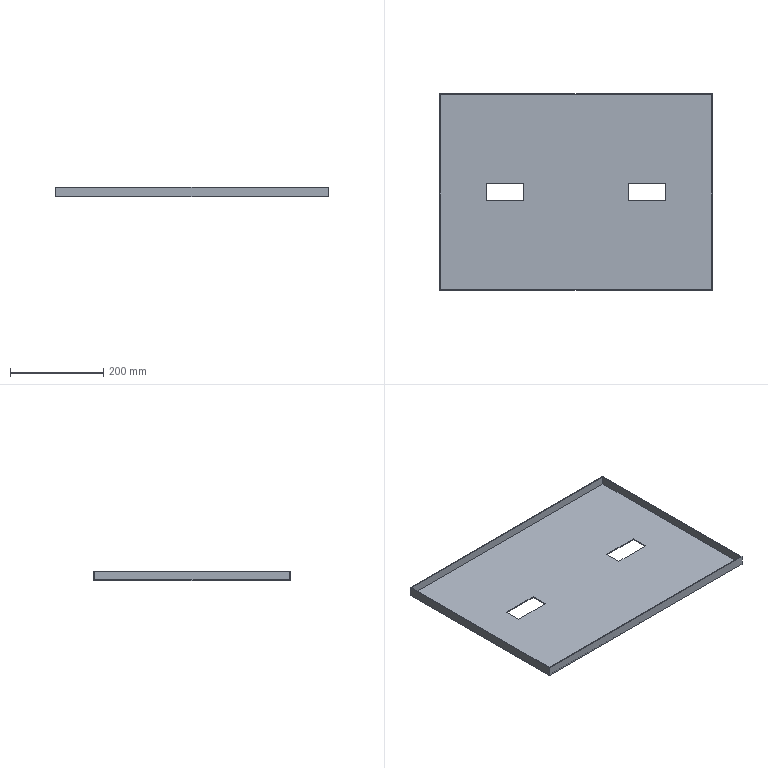Part | STEP file | Side sealing plate | 1 solid | 19 faces | box 585 x 421.75 x 20 mm | volume 553657 mm3 | plane 19
STEP:
#1=CARTESIAN_POINT('',(0.,0.,0.));
#2=DIRECTION('',(0.,0.,1.));
#3=DIRECTION('',(1.,0.,0.));
#4=AXIS2_PLACEMENT_3D('',#1,#2,#3);
#5=CARTESIAN_POINT('',(-292.5,-210.875,0.));
#6=VERTEX_POINT('',#5);
#7=CARTESIAN_POINT('',(292.5,-210.875,0.));
#8=VERTEX_POINT('',#7);
#9=CARTESIAN_POINT('',(0.,-210.875,0.));
#10=DIRECTION('',(1.,0.,0.));
#11=VECTOR('',#10,1.);
#12=LINE('',#9,#11);
#13=CARTESIAN_POINT('',(0.,0.,0.));
#14=DIRECTION('',(0.,0.,1.));
#15=DIRECTION('',(1.,0.,0.));
#16=AXIS2_PLACEMENT_3D('',#13,#14,#15);
#17=PLANE('',#16);
#18=CARTESIAN_POINT('',(0.,-210.875));
#19=DIRECTION('',(1.,0.));
#20=VECTOR('',#19,1.);
#21=LINE('',#18,#20);
#22=(GEOMETRIC_REPRESENTATION_CONTEXT(2)PARAMETRIC_REPRESENTATION_CONTEXT()REPRESENTATION_CONTEXT('',''));
#23=DEFINITIONAL_REPRESENTATION('',(#21),#22);
#24=PCURVE('',#17,#23);
#25=CARTESIAN_POINT('',(-292.5,-210.875,20.));
#26=DIRECTION('',(0.,1.,0.));
#27=DIRECTION('',(0.,0.,1.));
#28=AXIS2_PLACEMENT_3D('',#25,#26,#27);
#29=PLANE('',#28);
#30=CARTESIAN_POINT('',(-20.,292.5));
#31=DIRECTION('',(0.,1.));
#32=VECTOR('',#31,1.);
#33=LINE('',#30,#32);
#34=(GEOMETRIC_REPRESENTATION_CONTEXT(2)PARAMETRIC_REPRESENTATION_CONTEXT()REPRESENTATION_CONTEXT('',''));
#35=DEFINITIONAL_REPRESENTATION('',(#33),#34);
#36=PCURVE('',#29,#35);
#37=SURFACE_CURVE('',#12,(#24,#36),.PCURVE_S1.);
#38=EDGE_CURVE('',#6,#8,#37,.T.);
#39=ORIENTED_EDGE('',*,*,#38,.F.);
#40=CARTESIAN_POINT('',(-292.5,210.875,0.));
#41=VERTEX_POINT('',#40);
#42=CARTESIAN_POINT('',(-292.5,0.,0.));
#43=DIRECTION('',(0.,-1.,0.));
#44=VECTOR('',#43,1.);
#45=LINE('',#42,#44);
#46=CARTESIAN_POINT('',(-292.5,0.));
#47=DIRECTION('',(0.,-1.));
#48=VECTOR('',#47,1.);
#49=LINE('',#46,#48);
#50=(GEOMETRIC_REPRESENTATION_CONTEXT(2)PARAMETRIC_REPRESENTATION_CONTEXT()REPRESENTATION_CONTEXT('',''));
#51=DEFINITIONAL_REPRESENTATION('',(#49),#50);
#52=PCURVE('',#17,#51);
#53=CARTESIAN_POINT('',(-292.5,210.875,20.));
#54=DIRECTION('',(1.,0.,0.));
#55=DIRECTION('',(0.,1.,0.));
#56=AXIS2_PLACEMENT_3D('',#53,#54,#55);
#57=PLANE('',#56);
#58=CARTESIAN_POINT('',(-210.875,-20.));
#59=DIRECTION('',(-1.,0.));
#60=VECTOR('',#59,1.);
#61=LINE('',#58,#60);
#62=(GEOMETRIC_REPRESENTATION_CONTEXT(2)PARAMETRIC_REPRESENTATION_CONTEXT()REPRESENTATION_CONTEXT('',''));
#63=DEFINITIONAL_REPRESENTATION('',(#61),#62);
#64=PCURVE('',#57,#63);
#65=SURFACE_CURVE('',#45,(#52,#64),.PCURVE_S1.);
#66=EDGE_CURVE('',#41,#6,#65,.T.);
#67=ORIENTED_EDGE('',*,*,#66,.F.);
#68=CARTESIAN_POINT('',(292.5,210.875,0.));
#69=VERTEX_POINT('',#68);
#70=CARTESIAN_POINT('',(0.,210.875,0.));
#71=DIRECTION('',(-1.,0.,0.));
#72=VECTOR('',#71,1.);
#73=LINE('',#70,#72);
#74=CARTESIAN_POINT('',(0.,210.875));
#75=DIRECTION('',(-1.,0.));
#76=VECTOR('',#75,1.);
#77=LINE('',#74,#76);
#78=(GEOMETRIC_REPRESENTATION_CONTEXT(2)PARAMETRIC_REPRESENTATION_CONTEXT()REPRESENTATION_CONTEXT('',''));
#79=DEFINITIONAL_REPRESENTATION('',(#77),#78);
#80=PCURVE('',#17,#79);
#81=CARTESIAN_POINT('',(-292.5,210.875,20.));
#82=DIRECTION('',(0.,-1.,0.));
#83=DIRECTION('',(0.,0.,-1.));
#84=AXIS2_PLACEMENT_3D('',#81,#82,#83);
#85=PLANE('',#84);
#86=CARTESIAN_POINT('',(20.,292.5));
#87=DIRECTION('',(0.,-1.));
#88=VECTOR('',#87,1.);
#89=LINE('',#86,#88);
#90=(GEOMETRIC_REPRESENTATION_CONTEXT(2)PARAMETRIC_REPRESENTATION_CONTEXT()REPRESENTATION_CONTEXT('',''));
#91=DEFINITIONAL_REPRESENTATION('',(#89),#90);
#92=PCURVE('',#85,#91);
#93=SURFACE_CURVE('',#73,(#80,#92),.PCURVE_S1.);
#94=EDGE_CURVE('',#69,#41,#93,.T.);
#95=ORIENTED_EDGE('',*,*,#94,.F.);
#96=CARTESIAN_POINT('',(292.5,0.,0.));
#97=DIRECTION('',(0.,1.,0.));
#98=VECTOR('',#97,1.);
#99=LINE('',#96,#98);
#100=CARTESIAN_POINT('',(292.5,0.));
#101=DIRECTION('',(0.,1.));
#102=VECTOR('',#101,1.);
#103=LINE('',#100,#102);
#104=(GEOMETRIC_REPRESENTATION_CONTEXT(2)PARAMETRIC_REPRESENTATION_CONTEXT()REPRESENTATION_CONTEXT('',''));
#105=DEFINITIONAL_REPRESENTATION('',(#103),#104);
#106=PCURVE('',#17,#105);
#107=CARTESIAN_POINT('',(292.5,210.875,20.));
#108=DIRECTION('',(-1.,0.,0.));
#109=DIRECTION('',(0.,-1.,0.));
#110=AXIS2_PLACEMENT_3D('',#107,#108,#109);
#111=PLANE('',#110);
#112=CARTESIAN_POINT('',(210.875,-20.));
#113=DIRECTION('',(-1.,0.));
#114=VECTOR('',#113,1.);
#115=LINE('',#112,#114);
#116=(GEOMETRIC_REPRESENTATION_CONTEXT(2)PARAMETRIC_REPRESENTATION_CONTEXT()REPRESENTATION_CONTEXT('',''));
#117=DEFINITIONAL_REPRESENTATION('',(#115),#116);
#118=PCURVE('',#111,#117);
#119=SURFACE_CURVE('',#99,(#106,#118),.PCURVE_S1.);
#120=EDGE_CURVE('',#8,#69,#119,.T.);
#121=ORIENTED_EDGE('',*,*,#120,.F.);
#122=EDGE_LOOP('',(#39,#67,#95,#121));
#123=FACE_BOUND('',#122,.T.);
#124=CARTESIAN_POINT('',(111.5,-18.5,0.));
#125=VERTEX_POINT('',#124);
#126=CARTESIAN_POINT('',(111.5,18.5,0.));
#127=VERTEX_POINT('',#126);
#128=CARTESIAN_POINT('',(111.5,0.,0.));
#129=DIRECTION('',(0.,1.,0.));
#130=VECTOR('',#129,1.);
#131=LINE('',#128,#130);
#132=CARTESIAN_POINT('',(111.5,0.));
#133=DIRECTION('',(0.,1.));
#134=VECTOR('',#133,1.);
#135=LINE('',#132,#134);
#136=(GEOMETRIC_REPRESENTATION_CONTEXT(2)PARAMETRIC_REPRESENTATION_CONTEXT()REPRESENTATION_CONTEXT('',''));
#137=DEFINITIONAL_REPRESENTATION('',(#135),#136);
#138=PCURVE('',#17,#137);
#139=CARTESIAN_POINT('',(111.5,18.5,20.));
#140=DIRECTION('',(-1.,0.,0.));
#141=DIRECTION('',(0.,0.,1.));
#142=AXIS2_PLACEMENT_3D('',#139,#140,#141);
#143=PLANE('',#142);
#144=CARTESIAN_POINT('',(-20.,-18.5));
#145=DIRECTION('',(0.,1.));
#146=VECTOR('',#145,1.);
#147=LINE('',#144,#146);
#148=(GEOMETRIC_REPRESENTATION_CONTEXT(2)PARAMETRIC_REPRESENTATION_CONTEXT()REPRESENTATION_CONTEXT('',''));
#149=DEFINITIONAL_REPRESENTATION('',(#147),#148);
#150=PCURVE('',#143,#149);
#151=SURFACE_CURVE('',#131,(#138,#150),.PCURVE_S1.);
#152=EDGE_CURVE('',#125,#127,#151,.T.);
#153=ORIENTED_EDGE('',*,*,#152,.F.);
#154=CARTESIAN_POINT('',(192.5,-18.5,0.));
#155=VERTEX_POINT('',#154);
#156=CARTESIAN_POINT('',(0.,-18.5,0.));
#157=DIRECTION('',(-1.,0.,0.));
#158=VECTOR('',#157,1.);
#159=LINE('',#156,#158);
#160=CARTESIAN_POINT('',(0.,-18.5));
#161=DIRECTION('',(-1.,0.));
#162=VECTOR('',#161,1.);
#163=LINE('',#160,#162);
#164=(GEOMETRIC_REPRESENTATION_CONTEXT(2)PARAMETRIC_REPRESENTATION_CONTEXT()REPRESENTATION_CONTEXT('',''));
#165=DEFINITIONAL_REPRESENTATION('',(#163),#164);
#166=PCURVE('',#17,#165);
#167=CARTESIAN_POINT('',(192.5,-18.5,20.));
#168=DIRECTION('',(0.,-1.,0.));
#169=DIRECTION('',(0.,0.,-1.));
#170=AXIS2_PLACEMENT_3D('',#167,#168,#169);
#171=PLANE('',#170);
#172=CARTESIAN_POINT('',(20.,-192.5));
#173=DIRECTION('',(0.,-1.));
#174=VECTOR('',#173,1.);
#175=LINE('',#172,#174);
#176=(GEOMETRIC_REPRESENTATION_CONTEXT(2)PARAMETRIC_REPRESENTATION_CONTEXT()REPRESENTATION_CONTEXT('',''));
#177=DEFINITIONAL_REPRESENTATION('',(#175),#176);
#178=PCURVE('',#171,#177);
#179=SURFACE_CURVE('',#159,(#166,#178),.PCURVE_S1.);
#180=EDGE_CURVE('',#155,#125,#179,.T.);
#181=ORIENTED_EDGE('',*,*,#180,.F.);
#182=CARTESIAN_POINT('',(192.5,18.5,0.));
#183=VERTEX_POINT('',#182);
#184=CARTESIAN_POINT('',(192.5,0.,0.));
#185=DIRECTION('',(0.,-1.,0.));
#186=VECTOR('',#185,1.);
#187=LINE('',#184,#186);
#188=CARTESIAN_POINT('',(192.5,0.));
#189=DIRECTION('',(0.,-1.));
#190=VECTOR('',#189,1.);
#191=LINE('',#188,#190);
#192=(GEOMETRIC_REPRESENTATION_CONTEXT(2)PARAMETRIC_REPRESENTATION_CONTEXT()REPRESENTATION_CONTEXT('',''));
#193=DEFINITIONAL_REPRESENTATION('',(#191),#192);
#194=PCURVE('',#17,#193);
#195=CARTESIAN_POINT('',(192.5,18.5,20.));
#196=DIRECTION('',(1.,0.,0.));
#197=DIRECTION('',(0.,1.,0.));
#198=AXIS2_PLACEMENT_3D('',#195,#196,#197);
#199=PLANE('',#198);
#200=CARTESIAN_POINT('',(-18.5,-20.));
#201=DIRECTION('',(-1.,0.));
#202=VECTOR('',#201,1.);
#203=LINE('',#200,#202);
#204=(GEOMETRIC_REPRESENTATION_CONTEXT(2)PARAMETRIC_REPRESENTATION_CONTEXT()REPRESENTATION_CONTEXT('',''));
#205=DEFINITIONAL_REPRESENTATION('',(#203),#204);
#206=PCURVE('',#199,#205);
#207=SURFACE_CURVE('',#187,(#194,#206),.PCURVE_S1.);
#208=EDGE_CURVE('',#183,#155,#207,.T.);
#209=ORIENTED_EDGE('',*,*,#208,.F.);
#210=CARTESIAN_POINT('',(0.,18.5,0.));
#211=DIRECTION('',(1.,0.,0.));
#212=VECTOR('',#211,1.);
#213=LINE('',#210,#212);
#214=CARTESIAN_POINT('',(0.,18.5));
#215=DIRECTION('',(1.,0.));
#216=VECTOR('',#215,1.);
#217=LINE('',#214,#216);
#218=(GEOMETRIC_REPRESENTATION_CONTEXT(2)PARAMETRIC_REPRESENTATION_CONTEXT()REPRESENTATION_CONTEXT('',''));
#219=DEFINITIONAL_REPRESENTATION('',(#217),#218);
#220=PCURVE('',#17,#219);
#221=CARTESIAN_POINT('',(192.5,18.5,20.));
#222=DIRECTION('',(0.,1.,0.));
#223=DIRECTION('',(0.,0.,1.));
#224=AXIS2_PLACEMENT_3D('',#221,#222,#223);
#225=PLANE('',#224);
#226=CARTESIAN_POINT('',(-20.,-192.5));
#227=DIRECTION('',(0.,1.));
#228=VECTOR('',#227,1.);
#229=LINE('',#226,#228);
#230=(GEOMETRIC_REPRESENTATION_CONTEXT(2)PARAMETRIC_REPRESENTATION_CONTEXT()REPRESENTATION_CONTEXT('',''));
#231=DEFINITIONAL_REPRESENTATION('',(#229),#230);
#232=PCURVE('',#225,#231);
#233=SURFACE_CURVE('',#213,(#220,#232),.PCURVE_S1.);
#234=EDGE_CURVE('',#127,#183,#233,.T.);
#235=ORIENTED_EDGE('',*,*,#234,.F.);
#236=EDGE_LOOP('',(#153,#181,#209,#235));
#237=FACE_BOUND('',#236,.T.);
#238=CARTESIAN_POINT('',(-192.5,-18.5,0.));
#239=VERTEX_POINT('',#238);
#240=CARTESIAN_POINT('',(-192.5,18.5,0.));
#241=VERTEX_POINT('',#240);
#242=CARTESIAN_POINT('',(-192.5,0.,0.));
#243=DIRECTION('',(0.,1.,0.));
#244=VECTOR('',#243,1.);
#245=LINE('',#242,#244);
#246=CARTESIAN_POINT('',(-192.5,0.));
#247=DIRECTION('',(0.,1.));
#248=VECTOR('',#247,1.);
#249=LINE('',#246,#248);
#250=(GEOMETRIC_REPRESENTATION_CONTEXT(2)PARAMETRIC_REPRESENTATION_CONTEXT()REPRESENTATION_CONTEXT('',''));
#251=DEFINITIONAL_REPRESENTATION('',(#249),#250);
#252=PCURVE('',#17,#251);
#253=CARTESIAN_POINT('',(-192.5,18.5,20.));
#254=DIRECTION('',(-1.,0.,0.));
#255=DIRECTION('',(0.,0.,1.));
#256=AXIS2_PLACEMENT_3D('',#253,#254,#255);
#257=PLANE('',#256);
#258=CARTESIAN_POINT('',(-20.,-18.5));
#259=DIRECTION('',(0.,1.));
#260=VECTOR('',#259,1.);
#261=LINE('',#258,#260);
#262=(GEOMETRIC_REPRESENTATION_CONTEXT(2)PARAMETRIC_REPRESENTATION_CONTEXT()REPRESENTATION_CONTEXT('',''));
#263=DEFINITIONAL_REPRESENTATION('',(#261),#262);
#264=PCURVE('',#257,#263);
#265=SURFACE_CURVE('',#245,(#252,#264),.PCURVE_S1.);
#266=EDGE_CURVE('',#239,#241,#265,.T.);
#267=ORIENTED_EDGE('',*,*,#266,.F.);
#268=CARTESIAN_POINT('',(-111.5,-18.5,0.));
#269=VERTEX_POINT('',#268);
#270=CARTESIAN_POINT('',(0.,-18.5,0.));
#271=DIRECTION('',(-1.,0.,0.));
#272=VECTOR('',#271,1.);
#273=LINE('',#270,#272);
#274=CARTESIAN_POINT('',(0.,-18.5));
#275=DIRECTION('',(-1.,0.));
#276=VECTOR('',#275,1.);
#277=LINE('',#274,#276);
#278=(GEOMETRIC_REPRESENTATION_CONTEXT(2)PARAMETRIC_REPRESENTATION_CONTEXT()REPRESENTATION_CONTEXT('',''));
#279=DEFINITIONAL_REPRESENTATION('',(#277),#278);
#280=PCURVE('',#17,#279);
#281=CARTESIAN_POINT('',(-111.5,-18.5,20.));
#282=DIRECTION('',(0.,-1.,0.));
#283=DIRECTION('',(0.,0.,-1.));
#284=AXIS2_PLACEMENT_3D('',#281,#282,#283);
#285=PLANE('',#284);
#286=CARTESIAN_POINT('',(20.,111.5));
#287=DIRECTION('',(0.,-1.));
#288=VECTOR('',#287,1.);
#289=LINE('',#286,#288);
#290=(GEOMETRIC_REPRESENTATION_CONTEXT(2)PARAMETRIC_REPRESENTATION_CONTEXT()REPRESENTATION_CONTEXT('',''));
#291=DEFINITIONAL_REPRESENTATION('',(#289),#290);
#292=PCURVE('',#285,#291);
#293=SURFACE_CURVE('',#273,(#280,#292),.PCURVE_S1.);
#294=EDGE_CURVE('',#269,#239,#293,.T.);
#295=ORIENTED_EDGE('',*,*,#294,.F.);
#296=CARTESIAN_POINT('',(-111.5,18.5,0.));
#297=VERTEX_POINT('',#296);
#298=CARTESIAN_POINT('',(-111.5,0.,0.));
#299=DIRECTION('',(0.,-1.,0.));
#300=VECTOR('',#299,1.);
#301=LINE('',#298,#300);
#302=CARTESIAN_POINT('',(-111.5,0.));
#303=DIRECTION('',(0.,-1.));
#304=VECTOR('',#303,1.);
#305=LINE('',#302,#304);
#306=(GEOMETRIC_REPRESENTATION_CONTEXT(2)PARAMETRIC_REPRESENTATION_CONTEXT()REPRESENTATION_CONTEXT('',''));
#307=DEFINITIONAL_REPRESENTATION('',(#305),#306);
#308=PCURVE('',#17,#307);
#309=CARTESIAN_POINT('',(-111.5,18.5,20.));
#310=DIRECTION('',(1.,0.,0.));
#311=DIRECTION('',(0.,0.,-1.));
#312=AXIS2_PLACEMENT_3D('',#309,#310,#311);
#313=PLANE('',#312);
#314=CARTESIAN_POINT('',(20.,-18.5));
#315=DIRECTION('',(0.,-1.));
#316=VECTOR('',#315,1.);
#317=LINE('',#314,#316);
#318=(GEOMETRIC_REPRESENTATION_CONTEXT(2)PARAMETRIC_REPRESENTATION_CONTEXT()REPRESENTATION_CONTEXT('',''));
#319=DEFINITIONAL_REPRESENTATION('',(#317),#318);
#320=PCURVE('',#313,#319);
#321=SURFACE_CURVE('',#301,(#308,#320),.PCURVE_S1.);
#322=EDGE_CURVE('',#297,#269,#321,.T.);
#323=ORIENTED_EDGE('',*,*,#322,.F.);
#324=CARTESIAN_POINT('',(0.,18.5,0.));
#325=DIRECTION('',(1.,0.,0.));
#326=VECTOR('',#325,1.);
#327=LINE('',#324,#326);
#328=CARTESIAN_POINT('',(0.,18.5));
#329=DIRECTION('',(1.,0.));
#330=VECTOR('',#329,1.);
#331=LINE('',#328,#330);
#332=(GEOMETRIC_REPRESENTATION_CONTEXT(2)PARAMETRIC_REPRESENTATION_CONTEXT()REPRESENTATION_CONTEXT('',''));
#333=DEFINITIONAL_REPRESENTATION('',(#331),#332);
#334=PCURVE('',#17,#333);
#335=CARTESIAN_POINT('',(-111.5,18.5,20.));
#336=DIRECTION('',(0.,1.,0.));
#337=DIRECTION('',(-1.,0.,0.));
#338=AXIS2_PLACEMENT_3D('',#335,#336,#337);
#339=PLANE('',#338);
#340=CARTESIAN_POINT('',(-111.5,-20.));
#341=DIRECTION('',(-1.,0.));
#342=VECTOR('',#341,1.);
#343=LINE('',#340,#342);
#344=(GEOMETRIC_REPRESENTATION_CONTEXT(2)PARAMETRIC_REPRESENTATION_CONTEXT()REPRESENTATION_CONTEXT('',''));
#345=DEFINITIONAL_REPRESENTATION('',(#343),#344);
#346=PCURVE('',#339,#345);
#347=SURFACE_CURVE('',#327,(#334,#346),.PCURVE_S1.);
#348=EDGE_CURVE('',#241,#297,#347,.T.);
#349=ORIENTED_EDGE('',*,*,#348,.F.);
#350=EDGE_LOOP('',(#267,#295,#323,#349));
#351=FACE_BOUND('',#350,.T.);
#352=ADVANCED_FACE('',(#123,#237,#351),#17,.F.);
#353=CARTESIAN_POINT('',(292.5,210.875,20.));
#354=VERTEX_POINT('',#353);
#355=CARTESIAN_POINT('',(292.5,210.875,20.));
#356=DIRECTION('',(0.,0.,-1.));
#357=VECTOR('',#356,1.);
#358=LINE('',#355,#357);
#359=CARTESIAN_POINT('',(0.,0.));
#360=DIRECTION('',(0.,-1.));
#361=VECTOR('',#360,1.);
#362=LINE('',#359,#361);
#363=(GEOMETRIC_REPRESENTATION_CONTEXT(2)PARAMETRIC_REPRESENTATION_CONTEXT()REPRESENTATION_CONTEXT('',''));
#364=DEFINITIONAL_REPRESENTATION('',(#362),#363);
#365=PCURVE('',#111,#364);
#366=CARTESIAN_POINT('',(0.,585.));
#367=DIRECTION('',(1.,0.));
#368=VECTOR('',#367,1.);
#369=LINE('',#366,#368);
#370=(GEOMETRIC_REPRESENTATION_CONTEXT(2)PARAMETRIC_REPRESENTATION_CONTEXT()REPRESENTATION_CONTEXT('',''));
#371=DEFINITIONAL_REPRESENTATION('',(#369),#370);
#372=PCURVE('',#85,#371);
#373=SURFACE_CURVE('',#358,(#365,#372),.PCURVE_S1.);
#374=EDGE_CURVE('',#354,#69,#373,.T.);
#375=ORIENTED_EDGE('',*,*,#374,.F.);
#376=CARTESIAN_POINT('',(292.5,-210.875,20.));
#377=VERTEX_POINT('',#376);
#378=CARTESIAN_POINT('',(292.5,210.875,20.));
#379=DIRECTION('',(0.,1.,0.));
#380=VECTOR('',#379,1.);
#381=LINE('',#378,#380);
#382=CARTESIAN_POINT('',(0.,0.));
#383=DIRECTION('',(-1.,0.));
#384=VECTOR('',#383,1.);
#385=LINE('',#382,#384);
#386=(GEOMETRIC_REPRESENTATION_CONTEXT(2)PARAMETRIC_REPRESENTATION_CONTEXT()REPRESENTATION_CONTEXT('',''));
#387=DEFINITIONAL_REPRESENTATION('',(#385),#386);
#388=PCURVE('',#111,#387);
#389=CARTESIAN_POINT('',(0.,0.,20.));
#390=DIRECTION('',(0.,0.,1.));
#391=DIRECTION('',(1.,0.,0.));
#392=AXIS2_PLACEMENT_3D('',#389,#390,#391);
#393=PLANE('',#392);
#394=CARTESIAN_POINT('',(292.5,210.875));
#395=DIRECTION('',(0.,1.));
#396=VECTOR('',#395,1.);
#397=LINE('',#394,#396);
#398=(GEOMETRIC_REPRESENTATION_CONTEXT(2)PARAMETRIC_REPRESENTATION_CONTEXT()REPRESENTATION_CONTEXT('',''));
#399=DEFINITIONAL_REPRESENTATION('',(#397),#398);
#400=PCURVE('',#393,#399);
#401=SURFACE_CURVE('',#381,(#388,#400),.PCURVE_S1.);
#402=EDGE_CURVE('',#377,#354,#401,.T.);
#403=ORIENTED_EDGE('',*,*,#402,.F.);
#404=CARTESIAN_POINT('',(292.5,-210.875,20.));
#405=DIRECTION('',(0.,0.,1.));
#406=VECTOR('',#405,1.);
#407=LINE('',#404,#406);
#408=CARTESIAN_POINT('',(421.75,0.));
#409=DIRECTION('',(0.,1.));
#410=VECTOR('',#409,1.);
#411=LINE('',#408,#410);
#412=(GEOMETRIC_REPRESENTATION_CONTEXT(2)PARAMETRIC_REPRESENTATION_CONTEXT()REPRESENTATION_CONTEXT('',''));
#413=DEFINITIONAL_REPRESENTATION('',(#411),#412);
#414=PCURVE('',#111,#413);
#415=CARTESIAN_POINT('',(0.,585.));
#416=DIRECTION('',(1.,0.));
#417=VECTOR('',#416,1.);
#418=LINE('',#415,#417);
#419=(GEOMETRIC_REPRESENTATION_CONTEXT(2)PARAMETRIC_REPRESENTATION_CONTEXT()REPRESENTATION_CONTEXT('',''));
#420=DEFINITIONAL_REPRESENTATION('',(#418),#419);
#421=PCURVE('',#29,#420);
#422=SURFACE_CURVE('',#407,(#414,#421),.PCURVE_S1.);
#423=EDGE_CURVE('',#8,#377,#422,.T.);
#424=ORIENTED_EDGE('',*,*,#423,.F.);
#425=ORIENTED_EDGE('',*,*,#120,.T.);
#426=EDGE_LOOP('',(#375,#403,#424,#425));
#427=FACE_BOUND('',#426,.T.);
#428=ADVANCED_FACE('',(#427),#111,.F.);
#429=ORIENTED_EDGE('',*,*,#423,.T.);
#430=CARTESIAN_POINT('',(-292.5,-210.875,20.));
#431=VERTEX_POINT('',#430);
#432=CARTESIAN_POINT('',(-292.5,-210.875,20.));
#433=DIRECTION('',(1.,0.,0.));
#434=VECTOR('',#433,1.);
#435=LINE('',#432,#434);
#436=CARTESIAN_POINT('',(0.,0.));
#437=DIRECTION('',(0.,1.));
#438=VECTOR('',#437,1.);
#439=LINE('',#436,#438);
#440=(GEOMETRIC_REPRESENTATION_CONTEXT(2)PARAMETRIC_REPRESENTATION_CONTEXT()REPRESENTATION_CONTEXT('',''));
#441=DEFINITIONAL_REPRESENTATION('',(#439),#440);
#442=PCURVE('',#29,#441);
#443=CARTESIAN_POINT('',(-292.5,-210.875));
#444=DIRECTION('',(1.,0.));
#445=VECTOR('',#444,1.);
#446=LINE('',#443,#445);
#447=(GEOMETRIC_REPRESENTATION_CONTEXT(2)PARAMETRIC_REPRESENTATION_CONTEXT()REPRESENTATION_CONTEXT('',''));
#448=DEFINITIONAL_REPRESENTATION('',(#446),#447);
#449=PCURVE('',#393,#448);
#450=SURFACE_CURVE('',#435,(#442,#449),.PCURVE_S1.);
#451=EDGE_CURVE('',#431,#377,#450,.T.);
#452=ORIENTED_EDGE('',*,*,#451,.F.);
#453=CARTESIAN_POINT('',(-292.5,-210.875,20.));
#454=DIRECTION('',(0.,0.,1.));
#455=VECTOR('',#454,1.);
#456=LINE('',#453,#455);
#457=CARTESIAN_POINT('',(0.,0.));
#458=DIRECTION('',(1.,0.));
#459=VECTOR('',#458,1.);
#460=LINE('',#457,#459);
#461=(GEOMETRIC_REPRESENTATION_CONTEXT(2)PARAMETRIC_REPRESENTATION_CONTEXT()REPRESENTATION_CONTEXT('',''));
#462=DEFINITIONAL_REPRESENTATION('',(#460),#461);
#463=PCURVE('',#29,#462);
#464=CARTESIAN_POINT('',(-421.75,0.));
#465=DIRECTION('',(0.,1.));
#466=VECTOR('',#465,1.);
#467=LINE('',#464,#466);
#468=(GEOMETRIC_REPRESENTATION_CONTEXT(2)PARAMETRIC_REPRESENTATION_CONTEXT()REPRESENTATION_CONTEXT('',''));
#469=DEFINITIONAL_REPRESENTATION('',(#467),#468);
#470=PCURVE('',#57,#469);
#471=SURFACE_CURVE('',#456,(#463,#470),.PCURVE_S1.);
#472=EDGE_CURVE('',#6,#431,#471,.T.);
#473=ORIENTED_EDGE('',*,*,#472,.F.);
#474=ORIENTED_EDGE('',*,*,#38,.T.);
#475=EDGE_LOOP('',(#429,#452,#473,#474));
#476=FACE_BOUND('',#475,.T.);
#477=ADVANCED_FACE('',(#476),#29,.F.);
#478=ORIENTED_EDGE('',*,*,#472,.T.);
#479=CARTESIAN_POINT('',(-292.5,210.875,20.));
#480=VERTEX_POINT('',#479);
#481=CARTESIAN_POINT('',(-292.5,210.875,20.));
#482=DIRECTION('',(0.,-1.,0.));
#483=VECTOR('',#482,1.);
#484=LINE('',#481,#483);
#485=CARTESIAN_POINT('',(0.,0.));
#486=DIRECTION('',(-1.,0.));
#487=VECTOR('',#486,1.);
#488=LINE('',#485,#487);
#489=(GEOMETRIC_REPRESENTATION_CONTEXT(2)PARAMETRIC_REPRESENTATION_CONTEXT()REPRESENTATION_CONTEXT('',''));
#490=DEFINITIONAL_REPRESENTATION('',(#488),#489);
#491=PCURVE('',#57,#490);
#492=CARTESIAN_POINT('',(-292.5,210.875));
#493=DIRECTION('',(0.,-1.));
#494=VECTOR('',#493,1.);
#495=LINE('',#492,#494);
#496=(GEOMETRIC_REPRESENTATION_CONTEXT(2)PARAMETRIC_REPRESENTATION_CONTEXT()REPRESENTATION_CONTEXT('',''));
#497=DEFINITIONAL_REPRESENTATION('',(#495),#496);
#498=PCURVE('',#393,#497);
#499=SURFACE_CURVE('',#484,(#491,#498),.PCURVE_S1.);
#500=EDGE_CURVE('',#480,#431,#499,.T.);
#501=ORIENTED_EDGE('',*,*,#500,.F.);
#502=CARTESIAN_POINT('',(-292.5,210.875,20.));
#503=DIRECTION('',(0.,0.,1.));
#504=VECTOR('',#503,1.);
#505=LINE('',#502,#504);
#506=CARTESIAN_POINT('',(0.,0.));
#507=DIRECTION('',(0.,1.));
#508=VECTOR('',#507,1.);
#509=LINE('',#506,#508);
#510=(GEOMETRIC_REPRESENTATION_CONTEXT(2)PARAMETRIC_REPRESENTATION_CONTEXT()REPRESENTATION_CONTEXT('',''));
#511=DEFINITIONAL_REPRESENTATION('',(#509),#510);
#512=PCURVE('',#57,#511);
#513=CARTESIAN_POINT('',(0.,0.));
#514=DIRECTION('',(-1.,0.));
#515=VECTOR('',#514,1.);
#516=LINE('',#513,#515);
#517=(GEOMETRIC_REPRESENTATION_CONTEXT(2)PARAMETRIC_REPRESENTATION_CONTEXT()REPRESENTATION_CONTEXT('',''));
#518=DEFINITIONAL_REPRESENTATION('',(#516),#517);
#519=PCURVE('',#85,#518);
#520=SURFACE_CURVE('',#505,(#512,#519),.PCURVE_S1.);
#521=EDGE_CURVE('',#41,#480,#520,.T.);
#522=ORIENTED_EDGE('',*,*,#521,.F.);
#523=ORIENTED_EDGE('',*,*,#66,.T.);
#524=EDGE_LOOP('',(#478,#501,#522,#523));
#525=FACE_BOUND('',#524,.T.);
#526=ADVANCED_FACE('',(#525),#57,.F.);
#527=ORIENTED_EDGE('',*,*,#521,.T.);
#528=CARTESIAN_POINT('',(-292.5,210.875,20.));
#529=DIRECTION('',(-1.,0.,0.));
#530=VECTOR('',#529,1.);
#531=LINE('',#528,#530);
#532=CARTESIAN_POINT('',(0.,0.));
#533=DIRECTION('',(0.,-1.));
#534=VECTOR('',#533,1.);
#535=LINE('',#532,#534);
#536=(GEOMETRIC_REPRESENTATION_CONTEXT(2)PARAMETRIC_REPRESENTATION_CONTEXT()REPRESENTATION_CONTEXT('',''));
#537=DEFINITIONAL_REPRESENTATION('',(#535),#536);
#538=PCURVE('',#85,#537);
#539=CARTESIAN_POINT('',(-292.5,210.875));
#540=DIRECTION('',(-1.,0.));
#541=VECTOR('',#540,1.);
#542=LINE('',#539,#541);
#543=(GEOMETRIC_REPRESENTATION_CONTEXT(2)PARAMETRIC_REPRESENTATION_CONTEXT()REPRESENTATION_CONTEXT('',''));
#544=DEFINITIONAL_REPRESENTATION('',(#542),#543);
#545=PCURVE('',#393,#544);
#546=SURFACE_CURVE('',#531,(#538,#545),.PCURVE_S1.);
#547=EDGE_CURVE('',#354,#480,#546,.T.);
#548=ORIENTED_EDGE('',*,*,#547,.F.);
#549=ORIENTED_EDGE('',*,*,#374,.T.);
#550=ORIENTED_EDGE('',*,*,#94,.T.);
#551=EDGE_LOOP('',(#527,#548,#549,#550));
#552=FACE_BOUND('',#551,.T.);
#553=ADVANCED_FACE('',(#552),#85,.F.);
#554=CARTESIAN_POINT('',(111.5,18.5,2.));
#555=VERTEX_POINT('',#554);
#556=CARTESIAN_POINT('',(111.5,18.5,20.));
#557=DIRECTION('',(0.,0.,1.));
#558=VECTOR('',#557,1.);
#559=LINE('',#556,#558);
#560=CARTESIAN_POINT('',(0.,-81.));
#561=DIRECTION('',(1.,0.));
#562=VECTOR('',#561,1.);
#563=LINE('',#560,#562);
#564=(GEOMETRIC_REPRESENTATION_CONTEXT(2)PARAMETRIC_REPRESENTATION_CONTEXT()REPRESENTATION_CONTEXT('',''));
#565=DEFINITIONAL_REPRESENTATION('',(#563),#564);
#566=PCURVE('',#225,#565);
#567=CARTESIAN_POINT('',(0.,0.));
#568=DIRECTION('',(1.,0.));
#569=VECTOR('',#568,1.);
#570=LINE('',#567,#569);
#571=(GEOMETRIC_REPRESENTATION_CONTEXT(2)PARAMETRIC_REPRESENTATION_CONTEXT()REPRESENTATION_CONTEXT('',''));
#572=DEFINITIONAL_REPRESENTATION('',(#570),#571);
#573=PCURVE('',#143,#572);
#574=SURFACE_CURVE('',#559,(#566,#573),.PCURVE_S1.);
#575=EDGE_CURVE('',#127,#555,#574,.T.);
#576=ORIENTED_EDGE('',*,*,#575,.F.);
#577=ORIENTED_EDGE('',*,*,#234,.T.);
#578=CARTESIAN_POINT('',(192.5,18.5,2.));
#579=VERTEX_POINT('',#578);
#580=CARTESIAN_POINT('',(192.5,18.5,20.));
#581=DIRECTION('',(0.,0.,-1.));
#582=VECTOR('',#581,1.);
#583=LINE('',#580,#582);
#584=CARTESIAN_POINT('',(0.,0.));
#585=DIRECTION('',(-1.,0.));
#586=VECTOR('',#585,1.);
#587=LINE('',#584,#586);
#588=(GEOMETRIC_REPRESENTATION_CONTEXT(2)PARAMETRIC_REPRESENTATION_CONTEXT()REPRESENTATION_CONTEXT('',''));
#589=DEFINITIONAL_REPRESENTATION('',(#587),#588);
#590=PCURVE('',#225,#589);
#591=CARTESIAN_POINT('',(0.,0.));
#592=DIRECTION('',(0.,-1.));
#593=VECTOR('',#592,1.);
#594=LINE('',#591,#593);
#595=(GEOMETRIC_REPRESENTATION_CONTEXT(2)PARAMETRIC_REPRESENTATION_CONTEXT()REPRESENTATION_CONTEXT('',''));
#596=DEFINITIONAL_REPRESENTATION('',(#594),#595);
#597=PCURVE('',#199,#596);
#598=SURFACE_CURVE('',#583,(#590,#597),.PCURVE_S1.);
#599=EDGE_CURVE('',#579,#183,#598,.T.);
#600=ORIENTED_EDGE('',*,*,#599,.F.);
#601=CARTESIAN_POINT('',(192.5,18.5,2.));
#602=DIRECTION('',(1.,0.,0.));
#603=VECTOR('',#602,1.);
#604=LINE('',#601,#603);
#605=CARTESIAN_POINT('',(-18.,0.));
#606=DIRECTION('',(0.,1.));
#607=VECTOR('',#606,1.);
#608=LINE('',#605,#607);
#609=(GEOMETRIC_REPRESENTATION_CONTEXT(2)PARAMETRIC_REPRESENTATION_CONTEXT()REPRESENTATION_CONTEXT('',''));
#610=DEFINITIONAL_REPRESENTATION('',(#608),#609);
#611=PCURVE('',#225,#610);
#612=CARTESIAN_POINT('',(0.,0.,2.));
#613=DIRECTION('',(0.,0.,1.));
#614=DIRECTION('',(1.,0.,0.));
#615=AXIS2_PLACEMENT_3D('',#612,#613,#614);
#616=PLANE('',#615);
#617=CARTESIAN_POINT('',(192.5,18.5));
#618=DIRECTION('',(1.,0.));
#619=VECTOR('',#618,1.);
#620=LINE('',#617,#619);
#621=(GEOMETRIC_REPRESENTATION_CONTEXT(2)PARAMETRIC_REPRESENTATION_CONTEXT()REPRESENTATION_CONTEXT('',''));
#622=DEFINITIONAL_REPRESENTATION('',(#620),#621);
#623=PCURVE('',#616,#622);
#624=SURFACE_CURVE('',#604,(#611,#623),.PCURVE_S1.);
#625=EDGE_CURVE('',#555,#579,#624,.T.);
#626=ORIENTED_EDGE('',*,*,#625,.F.);
#627=EDGE_LOOP('',(#576,#577,#600,#626));
#628=FACE_BOUND('',#627,.T.);
#629=ADVANCED_FACE('',(#628),#225,.F.);
#630=CARTESIAN_POINT('',(111.5,-18.5,2.));
#631=VERTEX_POINT('',#630);
#632=CARTESIAN_POINT('',(111.5,-18.5,20.));
#633=DIRECTION('',(0.,0.,1.));
#634=VECTOR('',#633,1.);
#635=LINE('',#632,#634);
#636=CARTESIAN_POINT('',(0.,-37.));
#637=DIRECTION('',(1.,0.));
#638=VECTOR('',#637,1.);
#639=LINE('',#636,#638);
#640=(GEOMETRIC_REPRESENTATION_CONTEXT(2)PARAMETRIC_REPRESENTATION_CONTEXT()REPRESENTATION_CONTEXT('',''));
#641=DEFINITIONAL_REPRESENTATION('',(#639),#640);
#642=PCURVE('',#143,#641);
#643=CARTESIAN_POINT('',(0.,-81.));
#644=DIRECTION('',(-1.,0.));
#645=VECTOR('',#644,1.);
#646=LINE('',#643,#645);
#647=(GEOMETRIC_REPRESENTATION_CONTEXT(2)PARAMETRIC_REPRESENTATION_CONTEXT()REPRESENTATION_CONTEXT('',''));
#648=DEFINITIONAL_REPRESENTATION('',(#646),#647);
#649=PCURVE('',#171,#648);
#650=SURFACE_CURVE('',#635,(#642,#649),.PCURVE_S1.);
#651=EDGE_CURVE('',#125,#631,#650,.T.);
#652=ORIENTED_EDGE('',*,*,#651,.F.);
#653=ORIENTED_EDGE('',*,*,#152,.T.);
#654=ORIENTED_EDGE('',*,*,#575,.T.);
#655=CARTESIAN_POINT('',(111.5,18.5,2.));
#656=DIRECTION('',(0.,1.,0.));
#657=VECTOR('',#656,1.);
#658=LINE('',#655,#657);
#659=CARTESIAN_POINT('',(-18.,0.));
#660=DIRECTION('',(0.,1.));
#661=VECTOR('',#660,1.);
#662=LINE('',#659,#661);
#663=(GEOMETRIC_REPRESENTATION_CONTEXT(2)PARAMETRIC_REPRESENTATION_CONTEXT()REPRESENTATION_CONTEXT('',''));
#664=DEFINITIONAL_REPRESENTATION('',(#662),#663);
#665=PCURVE('',#143,#664);
#666=CARTESIAN_POINT('',(111.5,18.5));
#667=DIRECTION('',(0.,1.));
#668=VECTOR('',#667,1.);
#669=LINE('',#666,#668);
#670=(GEOMETRIC_REPRESENTATION_CONTEXT(2)PARAMETRIC_REPRESENTATION_CONTEXT()REPRESENTATION_CONTEXT('',''));
#671=DEFINITIONAL_REPRESENTATION('',(#669),#670);
#672=PCURVE('',#616,#671);
#673=SURFACE_CURVE('',#658,(#665,#672),.PCURVE_S1.);
#674=EDGE_CURVE('',#631,#555,#673,.T.);
#675=ORIENTED_EDGE('',*,*,#674,.F.);
#676=EDGE_LOOP('',(#652,#653,#654,#675));
#677=FACE_BOUND('',#676,.T.);
#678=ADVANCED_FACE('',(#677),#143,.F.);
#679=CARTESIAN_POINT('',(192.5,-18.5,2.));
#680=VERTEX_POINT('',#679);
#681=CARTESIAN_POINT('',(192.5,-18.5,20.));
#682=DIRECTION('',(0.,0.,1.));
#683=VECTOR('',#682,1.);
#684=LINE('',#681,#683);
#685=CARTESIAN_POINT('',(0.,0.));
#686=DIRECTION('',(-1.,0.));
#687=VECTOR('',#686,1.);
#688=LINE('',#685,#687);
#689=(GEOMETRIC_REPRESENTATION_CONTEXT(2)PARAMETRIC_REPRESENTATION_CONTEXT()REPRESENTATION_CONTEXT('',''));
#690=DEFINITIONAL_REPRESENTATION('',(#688),#689);
#691=PCURVE('',#171,#690);
#692=CARTESIAN_POINT('',(-37.,0.));
#693=DIRECTION('',(0.,1.));
#694=VECTOR('',#693,1.);
#695=LINE('',#692,#694);
#696=(GEOMETRIC_REPRESENTATION_CONTEXT(2)PARAMETRIC_REPRESENTATION_CONTEXT()REPRESENTATION_CONTEXT('',''));
#697=DEFINITIONAL_REPRESENTATION('',(#695),#696);
#698=PCURVE('',#199,#697);
#699=SURFACE_CURVE('',#684,(#691,#698),.PCURVE_S1.);
#700=EDGE_CURVE('',#155,#680,#699,.T.);
#701=ORIENTED_EDGE('',*,*,#700,.F.);
#702=ORIENTED_EDGE('',*,*,#180,.T.);
#703=ORIENTED_EDGE('',*,*,#651,.T.);
#704=CARTESIAN_POINT('',(192.5,-18.5,2.));
#705=DIRECTION('',(-1.,0.,0.));
#706=VECTOR('',#705,1.);
#707=LINE('',#704,#706);
#708=CARTESIAN_POINT('',(18.,0.));
#709=DIRECTION('',(0.,-1.));
#710=VECTOR('',#709,1.);
#711=LINE('',#708,#710);
#712=(GEOMETRIC_REPRESENTATION_CONTEXT(2)PARAMETRIC_REPRESENTATION_CONTEXT()REPRESENTATION_CONTEXT('',''));
#713=DEFINITIONAL_REPRESENTATION('',(#711),#712);
#714=PCURVE('',#171,#713);
#715=CARTESIAN_POINT('',(192.5,-18.5));
#716=DIRECTION('',(-1.,0.));
#717=VECTOR('',#716,1.);
#718=LINE('',#715,#717);
#719=(GEOMETRIC_REPRESENTATION_CONTEXT(2)PARAMETRIC_REPRESENTATION_CONTEXT()REPRESENTATION_CONTEXT('',''));
#720=DEFINITIONAL_REPRESENTATION('',(#718),#719);
#721=PCURVE('',#616,#720);
#722=SURFACE_CURVE('',#707,(#714,#721),.PCURVE_S1.);
#723=EDGE_CURVE('',#680,#631,#722,.T.);
#724=ORIENTED_EDGE('',*,*,#723,.F.);
#725=EDGE_LOOP('',(#701,#702,#703,#724));
#726=FACE_BOUND('',#725,.T.);
#727=ADVANCED_FACE('',(#726),#171,.F.);
#728=ORIENTED_EDGE('',*,*,#599,.T.);
#729=ORIENTED_EDGE('',*,*,#208,.T.);
#730=ORIENTED_EDGE('',*,*,#700,.T.);
#731=CARTESIAN_POINT('',(192.5,18.5,2.));
#732=DIRECTION('',(0.,-1.,0.));
#733=VECTOR('',#732,1.);
#734=LINE('',#731,#733);
#735=CARTESIAN_POINT('',(0.,-18.));
#736=DIRECTION('',(-1.,0.));
#737=VECTOR('',#736,1.);
#738=LINE('',#735,#737);
#739=(GEOMETRIC_REPRESENTATION_CONTEXT(2)PARAMETRIC_REPRESENTATION_CONTEXT()REPRESENTATION_CONTEXT('',''));
#740=DEFINITIONAL_REPRESENTATION('',(#738),#739);
#741=PCURVE('',#199,#740);
#742=CARTESIAN_POINT('',(192.5,18.5));
#743=DIRECTION('',(0.,-1.));
#744=VECTOR('',#743,1.);
#745=LINE('',#742,#744);
#746=(GEOMETRIC_REPRESENTATION_CONTEXT(2)PARAMETRIC_REPRESENTATION_CONTEXT()REPRESENTATION_CONTEXT('',''));
#747=DEFINITIONAL_REPRESENTATION('',(#745),#746);
#748=PCURVE('',#616,#747);
#749=SURFACE_CURVE('',#734,(#741,#748),.PCURVE_S1.);
#750=EDGE_CURVE('',#579,#680,#749,.T.);
#751=ORIENTED_EDGE('',*,*,#750,.F.);
#752=EDGE_LOOP('',(#728,#729,#730,#751));
#753=FACE_BOUND('',#752,.T.);
#754=ADVANCED_FACE('',(#753),#199,.F.);
#755=CARTESIAN_POINT('',(-192.5,18.5,2.));
#756=VERTEX_POINT('',#755);
#757=CARTESIAN_POINT('',(-192.5,18.5,20.));
#758=DIRECTION('',(0.,0.,1.));
#759=VECTOR('',#758,1.);
#760=LINE('',#757,#759);
#761=CARTESIAN_POINT('',(81.,0.));
#762=DIRECTION('',(0.,1.));
#763=VECTOR('',#762,1.);
#764=LINE('',#761,#763);
#765=(GEOMETRIC_REPRESENTATION_CONTEXT(2)PARAMETRIC_REPRESENTATION_CONTEXT()REPRESENTATION_CONTEXT('',''));
#766=DEFINITIONAL_REPRESENTATION('',(#764),#765);
#767=PCURVE('',#339,#766);
#768=CARTESIAN_POINT('',(0.,0.));
#769=DIRECTION('',(1.,0.));
#770=VECTOR('',#769,1.);
#771=LINE('',#768,#770);
#772=(GEOMETRIC_REPRESENTATION_CONTEXT(2)PARAMETRIC_REPRESENTATION_CONTEXT()REPRESENTATION_CONTEXT('',''));
#773=DEFINITIONAL_REPRESENTATION('',(#771),#772);
#774=PCURVE('',#257,#773);
#775=SURFACE_CURVE('',#760,(#767,#774),.PCURVE_S1.);
#776=EDGE_CURVE('',#241,#756,#775,.T.);
#777=ORIENTED_EDGE('',*,*,#776,.F.);
#778=ORIENTED_EDGE('',*,*,#348,.T.);
#779=CARTESIAN_POINT('',(-111.5,18.5,2.));
#780=VERTEX_POINT('',#779);
#781=CARTESIAN_POINT('',(-111.5,18.5,20.));
#782=DIRECTION('',(0.,0.,-1.));
#783=VECTOR('',#782,1.);
#784=LINE('',#781,#783);
#785=CARTESIAN_POINT('',(0.,0.));
#786=DIRECTION('',(0.,-1.));
#787=VECTOR('',#786,1.);
#788=LINE('',#785,#787);
#789=(GEOMETRIC_REPRESENTATION_CONTEXT(2)PARAMETRIC_REPRESENTATION_CONTEXT()REPRESENTATION_CONTEXT('',''));
#790=DEFINITIONAL_REPRESENTATION('',(#788),#789);
#791=PCURVE('',#339,#790);
#792=CARTESIAN_POINT('',(0.,0.));
#793=DIRECTION('',(1.,0.));
#794=VECTOR('',#793,1.);
#795=LINE('',#792,#794);
#796=(GEOMETRIC_REPRESENTATION_CONTEXT(2)PARAMETRIC_REPRESENTATION_CONTEXT()REPRESENTATION_CONTEXT('',''));
#797=DEFINITIONAL_REPRESENTATION('',(#795),#796);
#798=PCURVE('',#313,#797);
#799=SURFACE_CURVE('',#784,(#791,#798),.PCURVE_S1.);
#800=EDGE_CURVE('',#780,#297,#799,.T.);
#801=ORIENTED_EDGE('',*,*,#800,.F.);
#802=CARTESIAN_POINT('',(-111.5,18.5,2.));
#803=DIRECTION('',(1.,0.,0.));
#804=VECTOR('',#803,1.);
#805=LINE('',#802,#804);
#806=CARTESIAN_POINT('',(0.,-18.));
#807=DIRECTION('',(-1.,0.));
#808=VECTOR('',#807,1.);
#809=LINE('',#806,#808);
#810=(GEOMETRIC_REPRESENTATION_CONTEXT(2)PARAMETRIC_REPRESENTATION_CONTEXT()REPRESENTATION_CONTEXT('',''));
#811=DEFINITIONAL_REPRESENTATION('',(#809),#810);
#812=PCURVE('',#339,#811);
#813=CARTESIAN_POINT('',(-111.5,18.5));
#814=DIRECTION('',(1.,0.));
#815=VECTOR('',#814,1.);
#816=LINE('',#813,#815);
#817=(GEOMETRIC_REPRESENTATION_CONTEXT(2)PARAMETRIC_REPRESENTATION_CONTEXT()REPRESENTATION_CONTEXT('',''));
#818=DEFINITIONAL_REPRESENTATION('',(#816),#817);
#819=PCURVE('',#616,#818);
#820=SURFACE_CURVE('',#805,(#812,#819),.PCURVE_S1.);
#821=EDGE_CURVE('',#756,#780,#820,.T.);
#822=ORIENTED_EDGE('',*,*,#821,.F.);
#823=EDGE_LOOP('',(#777,#778,#801,#822));
#824=FACE_BOUND('',#823,.T.);
#825=ADVANCED_FACE('',(#824),#339,.F.);
#826=CARTESIAN_POINT('',(-192.5,-18.5,2.));
#827=VERTEX_POINT('',#826);
#828=CARTESIAN_POINT('',(-192.5,-18.5,20.));
#829=DIRECTION('',(0.,0.,1.));
#830=VECTOR('',#829,1.);
#831=LINE('',#828,#830);
#832=CARTESIAN_POINT('',(0.,-37.));
#833=DIRECTION('',(1.,0.));
#834=VECTOR('',#833,1.);
#835=LINE('',#832,#834);
#836=(GEOMETRIC_REPRESENTATION_CONTEXT(2)PARAMETRIC_REPRESENTATION_CONTEXT()REPRESENTATION_CONTEXT('',''));
#837=DEFINITIONAL_REPRESENTATION('',(#835),#836);
#838=PCURVE('',#257,#837);
#839=CARTESIAN_POINT('',(0.,-81.));
#840=DIRECTION('',(-1.,0.));
#841=VECTOR('',#840,1.);
#842=LINE('',#839,#841);
#843=(GEOMETRIC_REPRESENTATION_CONTEXT(2)PARAMETRIC_REPRESENTATION_CONTEXT()REPRESENTATION_CONTEXT('',''));
#844=DEFINITIONAL_REPRESENTATION('',(#842),#843);
#845=PCURVE('',#285,#844);
#846=SURFACE_CURVE('',#831,(#838,#845),.PCURVE_S1.);
#847=EDGE_CURVE('',#239,#827,#846,.T.);
#848=ORIENTED_EDGE('',*,*,#847,.F.);
#849=ORIENTED_EDGE('',*,*,#266,.T.);
#850=ORIENTED_EDGE('',*,*,#776,.T.);
#851=CARTESIAN_POINT('',(-192.5,18.5,2.));
#852=DIRECTION('',(0.,1.,0.));
#853=VECTOR('',#852,1.);
#854=LINE('',#851,#853);
#855=CARTESIAN_POINT('',(-18.,0.));
#856=DIRECTION('',(0.,1.));
#857=VECTOR('',#856,1.);
#858=LINE('',#855,#857);
#859=(GEOMETRIC_REPRESENTATION_CONTEXT(2)PARAMETRIC_REPRESENTATION_CONTEXT()REPRESENTATION_CONTEXT('',''));
#860=DEFINITIONAL_REPRESENTATION('',(#858),#859);
#861=PCURVE('',#257,#860);
#862=CARTESIAN_POINT('',(-192.5,18.5));
#863=DIRECTION('',(0.,1.));
#864=VECTOR('',#863,1.);
#865=LINE('',#862,#864);
#866=(GEOMETRIC_REPRESENTATION_CONTEXT(2)PARAMETRIC_REPRESENTATION_CONTEXT()REPRESENTATION_CONTEXT('',''));
#867=DEFINITIONAL_REPRESENTATION('',(#865),#866);
#868=PCURVE('',#616,#867);
#869=SURFACE_CURVE('',#854,(#861,#868),.PCURVE_S1.);
#870=EDGE_CURVE('',#827,#756,#869,.T.);
#871=ORIENTED_EDGE('',*,*,#870,.F.);
#872=EDGE_LOOP('',(#848,#849,#850,#871));
#873=FACE_BOUND('',#872,.T.);
#874=ADVANCED_FACE('',(#873),#257,.F.);
#875=CARTESIAN_POINT('',(-111.5,-18.5,2.));
#876=VERTEX_POINT('',#875);
#877=CARTESIAN_POINT('',(-111.5,-18.5,20.));
#878=DIRECTION('',(0.,0.,1.));
#879=VECTOR('',#878,1.);
#880=LINE('',#877,#879);
#881=CARTESIAN_POINT('',(0.,0.));
#882=DIRECTION('',(-1.,0.));
#883=VECTOR('',#882,1.);
#884=LINE('',#881,#883);
#885=(GEOMETRIC_REPRESENTATION_CONTEXT(2)PARAMETRIC_REPRESENTATION_CONTEXT()REPRESENTATION_CONTEXT('',''));
#886=DEFINITIONAL_REPRESENTATION('',(#884),#885);
#887=PCURVE('',#285,#886);
#888=CARTESIAN_POINT('',(0.,-37.));
#889=DIRECTION('',(-1.,0.));
#890=VECTOR('',#889,1.);
#891=LINE('',#888,#890);
#892=(GEOMETRIC_REPRESENTATION_CONTEXT(2)PARAMETRIC_REPRESENTATION_CONTEXT()REPRESENTATION_CONTEXT('',''));
#893=DEFINITIONAL_REPRESENTATION('',(#891),#892);
#894=PCURVE('',#313,#893);
#895=SURFACE_CURVE('',#880,(#887,#894),.PCURVE_S1.);
#896=EDGE_CURVE('',#269,#876,#895,.T.);
#897=ORIENTED_EDGE('',*,*,#896,.F.);
#898=ORIENTED_EDGE('',*,*,#294,.T.);
#899=ORIENTED_EDGE('',*,*,#847,.T.);
#900=CARTESIAN_POINT('',(-111.5,-18.5,2.));
#901=DIRECTION('',(-1.,0.,0.));
#902=VECTOR('',#901,1.);
#903=LINE('',#900,#902);
#904=CARTESIAN_POINT('',(18.,0.));
#905=DIRECTION('',(0.,-1.));
#906=VECTOR('',#905,1.);
#907=LINE('',#904,#906);
#908=(GEOMETRIC_REPRESENTATION_CONTEXT(2)PARAMETRIC_REPRESENTATION_CONTEXT()REPRESENTATION_CONTEXT('',''));
#909=DEFINITIONAL_REPRESENTATION('',(#907),#908);
#910=PCURVE('',#285,#909);
#911=CARTESIAN_POINT('',(-111.5,-18.5));
#912=DIRECTION('',(-1.,0.));
#913=VECTOR('',#912,1.);
#914=LINE('',#911,#913);
#915=(GEOMETRIC_REPRESENTATION_CONTEXT(2)PARAMETRIC_REPRESENTATION_CONTEXT()REPRESENTATION_CONTEXT('',''));
#916=DEFINITIONAL_REPRESENTATION('',(#914),#915);
#917=PCURVE('',#616,#916);
#918=SURFACE_CURVE('',#903,(#910,#917),.PCURVE_S1.);
#919=EDGE_CURVE('',#876,#827,#918,.T.);
#920=ORIENTED_EDGE('',*,*,#919,.F.);
#921=EDGE_LOOP('',(#897,#898,#899,#920));
#922=FACE_BOUND('',#921,.T.);
#923=ADVANCED_FACE('',(#922),#285,.F.);
#924=ORIENTED_EDGE('',*,*,#800,.T.);
#925=ORIENTED_EDGE('',*,*,#322,.T.);
#926=ORIENTED_EDGE('',*,*,#896,.T.);
#927=CARTESIAN_POINT('',(-111.5,18.5,2.));
#928=DIRECTION('',(0.,-1.,0.));
#929=VECTOR('',#928,1.);
#930=LINE('',#927,#929);
#931=CARTESIAN_POINT('',(18.,0.));
#932=DIRECTION('',(0.,-1.));
#933=VECTOR('',#932,1.);
#934=LINE('',#931,#933);
#935=(GEOMETRIC_REPRESENTATION_CONTEXT(2)PARAMETRIC_REPRESENTATION_CONTEXT()REPRESENTATION_CONTEXT('',''));
#936=DEFINITIONAL_REPRESENTATION('',(#934),#935);
#937=PCURVE('',#313,#936);
#938=CARTESIAN_POINT('',(-111.5,18.5));
#939=DIRECTION('',(0.,-1.));
#940=VECTOR('',#939,1.);
#941=LINE('',#938,#940);
#942=(GEOMETRIC_REPRESENTATION_CONTEXT(2)PARAMETRIC_REPRESENTATION_CONTEXT()REPRESENTATION_CONTEXT('',''));
#943=DEFINITIONAL_REPRESENTATION('',(#941),#942);
#944=PCURVE('',#616,#943);
#945=SURFACE_CURVE('',#930,(#937,#944),.PCURVE_S1.);
#946=EDGE_CURVE('',#780,#876,#945,.T.);
#947=ORIENTED_EDGE('',*,*,#946,.F.);
#948=EDGE_LOOP('',(#924,#925,#926,#947));
#949=FACE_BOUND('',#948,.T.);
#950=ADVANCED_FACE('',(#949),#313,.F.);
#951=ORIENTED_EDGE('',*,*,#500,.T.);
#952=ORIENTED_EDGE('',*,*,#451,.T.);
#953=ORIENTED_EDGE('',*,*,#402,.T.);
#954=ORIENTED_EDGE('',*,*,#547,.T.);
#955=EDGE_LOOP('',(#951,#952,#953,#954));
#956=FACE_BOUND('',#955,.T.);
#957=CARTESIAN_POINT('',(-290.5,-208.875,20.));
#958=VERTEX_POINT('',#957);
#959=CARTESIAN_POINT('',(-290.5,208.875,20.));
#960=VERTEX_POINT('',#959);
#961=CARTESIAN_POINT('',(-290.5,0.,20.));
#962=DIRECTION('',(0.,1.,0.));
#963=VECTOR('',#962,1.);
#964=LINE('',#961,#963);
#965=CARTESIAN_POINT('',(-290.5,0.));
#966=DIRECTION('',(0.,1.));
#967=VECTOR('',#966,1.);
#968=LINE('',#965,#967);
#969=(GEOMETRIC_REPRESENTATION_CONTEXT(2)PARAMETRIC_REPRESENTATION_CONTEXT()REPRESENTATION_CONTEXT('',''));
#970=DEFINITIONAL_REPRESENTATION('',(#968),#969);
#971=PCURVE('',#393,#970);
#972=CARTESIAN_POINT('',(-290.5,210.875,20.));
#973=DIRECTION('',(1.,0.,0.));
#974=DIRECTION('',(0.,1.,0.));
#975=AXIS2_PLACEMENT_3D('',#972,#973,#974);
#976=PLANE('',#975);
#977=CARTESIAN_POINT('',(-210.875,0.));
#978=DIRECTION('',(1.,0.));
#979=VECTOR('',#978,1.);
#980=LINE('',#977,#979);
#981=(GEOMETRIC_REPRESENTATION_CONTEXT(2)PARAMETRIC_REPRESENTATION_CONTEXT()REPRESENTATION_CONTEXT('',''));
#982=DEFINITIONAL_REPRESENTATION('',(#980),#981);
#983=PCURVE('',#976,#982);
#984=SURFACE_CURVE('',#964,(#971,#983),.PCURVE_S1.);
#985=EDGE_CURVE('',#958,#960,#984,.T.);
#986=ORIENTED_EDGE('',*,*,#985,.T.);
#987=CARTESIAN_POINT('',(290.5,208.875,20.));
#988=VERTEX_POINT('',#987);
#989=CARTESIAN_POINT('',(0.,208.875,20.));
#990=DIRECTION('',(1.,0.,0.));
#991=VECTOR('',#990,1.);
#992=LINE('',#989,#991);
#993=CARTESIAN_POINT('',(0.,208.875));
#994=DIRECTION('',(1.,0.));
#995=VECTOR('',#994,1.);
#996=LINE('',#993,#995);
#997=(GEOMETRIC_REPRESENTATION_CONTEXT(2)PARAMETRIC_REPRESENTATION_CONTEXT()REPRESENTATION_CONTEXT('',''));
#998=DEFINITIONAL_REPRESENTATION('',(#996),#997);
#999=PCURVE('',#393,#998);
#1000=CARTESIAN_POINT('',(-292.5,208.875,20.));
#1001=DIRECTION('',(0.,-1.,0.));
#1002=DIRECTION('',(0.,0.,-1.));
#1003=AXIS2_PLACEMENT_3D('',#1000,#1001,#1002);
#1004=PLANE('',#1003);
#1005=CARTESIAN_POINT('',(0.,292.5));
#1006=DIRECTION('',(0.,1.));
#1007=VECTOR('',#1006,1.);
#1008=LINE('',#1005,#1007);
#1009=(GEOMETRIC_REPRESENTATION_CONTEXT(2)PARAMETRIC_REPRESENTATION_CONTEXT()REPRESENTATION_CONTEXT('',''));
#1010=DEFINITIONAL_REPRESENTATION('',(#1008),#1009);
#1011=PCURVE('',#1004,#1010);
#1012=SURFACE_CURVE('',#992,(#999,#1011),.PCURVE_S1.);
#1013=EDGE_CURVE('',#960,#988,#1012,.T.);
#1014=ORIENTED_EDGE('',*,*,#1013,.T.);
#1015=CARTESIAN_POINT('',(290.5,-208.875,20.));
#1016=VERTEX_POINT('',#1015);
#1017=CARTESIAN_POINT('',(290.5,0.,20.));
#1018=DIRECTION('',(0.,-1.,0.));
#1019=VECTOR('',#1018,1.);
#1020=LINE('',#1017,#1019);
#1021=CARTESIAN_POINT('',(290.5,0.));
#1022=DIRECTION('',(0.,-1.));
#1023=VECTOR('',#1022,1.);
#1024=LINE('',#1021,#1023);
#1025=(GEOMETRIC_REPRESENTATION_CONTEXT(2)PARAMETRIC_REPRESENTATION_CONTEXT()REPRESENTATION_CONTEXT('',''));
#1026=DEFINITIONAL_REPRESENTATION('',(#1024),#1025);
#1027=PCURVE('',#393,#1026);
#1028=CARTESIAN_POINT('',(290.5,210.875,20.));
#1029=DIRECTION('',(-1.,0.,0.));
#1030=DIRECTION('',(0.,-1.,0.));
#1031=AXIS2_PLACEMENT_3D('',#1028,#1029,#1030);
#1032=PLANE('',#1031);
#1033=CARTESIAN_POINT('',(210.875,0.));
#1034=DIRECTION('',(1.,0.));
#1035=VECTOR('',#1034,1.);
#1036=LINE('',#1033,#1035);
#1037=(GEOMETRIC_REPRESENTATION_CONTEXT(2)PARAMETRIC_REPRESENTATION_CONTEXT()REPRESENTATION_CONTEXT('',''));
#1038=DEFINITIONAL_REPRESENTATION('',(#1036),#1037);
#1039=PCURVE('',#1032,#1038);
#1040=SURFACE_CURVE('',#1020,(#1027,#1039),.PCURVE_S1.);
#1041=EDGE_CURVE('',#988,#1016,#1040,.T.);
#1042=ORIENTED_EDGE('',*,*,#1041,.T.);
#1043=CARTESIAN_POINT('',(0.,-208.875,20.));
#1044=DIRECTION('',(-1.,0.,0.));
#1045=VECTOR('',#1044,1.);
#1046=LINE('',#1043,#1045);
#1047=CARTESIAN_POINT('',(0.,-208.875));
#1048=DIRECTION('',(-1.,0.));
#1049=VECTOR('',#1048,1.);
#1050=LINE('',#1047,#1049);
#1051=(GEOMETRIC_REPRESENTATION_CONTEXT(2)PARAMETRIC_REPRESENTATION_CONTEXT()REPRESENTATION_CONTEXT('',''));
#1052=DEFINITIONAL_REPRESENTATION('',(#1050),#1051);
#1053=PCURVE('',#393,#1052);
#1054=CARTESIAN_POINT('',(-292.5,-208.875,20.));
#1055=DIRECTION('',(0.,1.,0.));
#1056=DIRECTION('',(0.,0.,1.));
#1057=AXIS2_PLACEMENT_3D('',#1054,#1055,#1056);
#1058=PLANE('',#1057);
#1059=CARTESIAN_POINT('',(0.,292.5));
#1060=DIRECTION('',(0.,-1.));
#1061=VECTOR('',#1060,1.);
#1062=LINE('',#1059,#1061);
#1063=(GEOMETRIC_REPRESENTATION_CONTEXT(2)PARAMETRIC_REPRESENTATION_CONTEXT()REPRESENTATION_CONTEXT('',''));
#1064=DEFINITIONAL_REPRESENTATION('',(#1062),#1063);
#1065=PCURVE('',#1058,#1064);
#1066=SURFACE_CURVE('',#1046,(#1053,#1065),.PCURVE_S1.);
#1067=EDGE_CURVE('',#1016,#958,#1066,.T.);
#1068=ORIENTED_EDGE('',*,*,#1067,.T.);
#1069=EDGE_LOOP('',(#986,#1014,#1042,#1068));
#1070=FACE_BOUND('',#1069,.T.);
#1071=ADVANCED_FACE('',(#956,#1070),#393,.T.);
#1072=CARTESIAN_POINT('',(-290.5,208.875,2.));
#1073=VERTEX_POINT('',#1072);
#1074=CARTESIAN_POINT('',(-290.5,-208.875,2.));
#1075=VERTEX_POINT('',#1074);
#1076=CARTESIAN_POINT('',(-290.5,0.,2.));
#1077=DIRECTION('',(0.,-1.,0.));
#1078=VECTOR('',#1077,1.);
#1079=LINE('',#1076,#1078);
#1080=CARTESIAN_POINT('',(-290.5,0.));
#1081=DIRECTION('',(0.,-1.));
#1082=VECTOR('',#1081,1.);
#1083=LINE('',#1080,#1082);
#1084=(GEOMETRIC_REPRESENTATION_CONTEXT(2)PARAMETRIC_REPRESENTATION_CONTEXT()REPRESENTATION_CONTEXT('',''));
#1085=DEFINITIONAL_REPRESENTATION('',(#1083),#1084);
#1086=PCURVE('',#616,#1085);
#1087=CARTESIAN_POINT('',(-210.875,-18.));
#1088=DIRECTION('',(-1.,0.));
#1089=VECTOR('',#1088,1.);
#1090=LINE('',#1087,#1089);
#1091=(GEOMETRIC_REPRESENTATION_CONTEXT(2)PARAMETRIC_REPRESENTATION_CONTEXT()REPRESENTATION_CONTEXT('',''));
#1092=DEFINITIONAL_REPRESENTATION('',(#1090),#1091);
#1093=PCURVE('',#976,#1092);
#1094=SURFACE_CURVE('',#1079,(#1086,#1093),.PCURVE_S1.);
#1095=EDGE_CURVE('',#1073,#1075,#1094,.T.);
#1096=ORIENTED_EDGE('',*,*,#1095,.T.);
#1097=CARTESIAN_POINT('',(290.5,-208.875,2.));
#1098=VERTEX_POINT('',#1097);
#1099=CARTESIAN_POINT('',(0.,-208.875,2.));
#1100=DIRECTION('',(1.,0.,0.));
#1101=VECTOR('',#1100,1.);
#1102=LINE('',#1099,#1101);
#1103=CARTESIAN_POINT('',(0.,-208.875));
#1104=DIRECTION('',(1.,0.));
#1105=VECTOR('',#1104,1.);
#1106=LINE('',#1103,#1105);
#1107=(GEOMETRIC_REPRESENTATION_CONTEXT(2)PARAMETRIC_REPRESENTATION_CONTEXT()REPRESENTATION_CONTEXT('',''));
#1108=DEFINITIONAL_REPRESENTATION('',(#1106),#1107);
#1109=PCURVE('',#616,#1108);
#1110=CARTESIAN_POINT('',(-18.,292.5));
#1111=DIRECTION('',(0.,1.));
#1112=VECTOR('',#1111,1.);
#1113=LINE('',#1110,#1112);
#1114=(GEOMETRIC_REPRESENTATION_CONTEXT(2)PARAMETRIC_REPRESENTATION_CONTEXT()REPRESENTATION_CONTEXT('',''));
#1115=DEFINITIONAL_REPRESENTATION('',(#1113),#1114);
#1116=PCURVE('',#1058,#1115);
#1117=SURFACE_CURVE('',#1102,(#1109,#1116),.PCURVE_S1.);
#1118=EDGE_CURVE('',#1075,#1098,#1117,.T.);
#1119=ORIENTED_EDGE('',*,*,#1118,.T.);
#1120=CARTESIAN_POINT('',(290.5,208.875,2.));
#1121=VERTEX_POINT('',#1120);
#1122=CARTESIAN_POINT('',(290.5,0.,2.));
#1123=DIRECTION('',(0.,1.,0.));
#1124=VECTOR('',#1123,1.);
#1125=LINE('',#1122,#1124);
#1126=CARTESIAN_POINT('',(290.5,0.));
#1127=DIRECTION('',(0.,1.));
#1128=VECTOR('',#1127,1.);
#1129=LINE('',#1126,#1128);
#1130=(GEOMETRIC_REPRESENTATION_CONTEXT(2)PARAMETRIC_REPRESENTATION_CONTEXT()REPRESENTATION_CONTEXT('',''));
#1131=DEFINITIONAL_REPRESENTATION('',(#1129),#1130);
#1132=PCURVE('',#616,#1131);
#1133=CARTESIAN_POINT('',(210.875,-18.));
#1134=DIRECTION('',(-1.,0.));
#1135=VECTOR('',#1134,1.);
#1136=LINE('',#1133,#1135);
#1137=(GEOMETRIC_REPRESENTATION_CONTEXT(2)PARAMETRIC_REPRESENTATION_CONTEXT()REPRESENTATION_CONTEXT('',''));
#1138=DEFINITIONAL_REPRESENTATION('',(#1136),#1137);
#1139=PCURVE('',#1032,#1138);
#1140=SURFACE_CURVE('',#1125,(#1132,#1139),.PCURVE_S1.);
#1141=EDGE_CURVE('',#1098,#1121,#1140,.T.);
#1142=ORIENTED_EDGE('',*,*,#1141,.T.);
#1143=CARTESIAN_POINT('',(0.,208.875,2.));
#1144=DIRECTION('',(-1.,0.,0.));
#1145=VECTOR('',#1144,1.);
#1146=LINE('',#1143,#1145);
#1147=CARTESIAN_POINT('',(0.,208.875));
#1148=DIRECTION('',(-1.,0.));
#1149=VECTOR('',#1148,1.);
#1150=LINE('',#1147,#1149);
#1151=(GEOMETRIC_REPRESENTATION_CONTEXT(2)PARAMETRIC_REPRESENTATION_CONTEXT()REPRESENTATION_CONTEXT('',''));
#1152=DEFINITIONAL_REPRESENTATION('',(#1150),#1151);
#1153=PCURVE('',#616,#1152);
#1154=CARTESIAN_POINT('',(18.,292.5));
#1155=DIRECTION('',(0.,-1.));
#1156=VECTOR('',#1155,1.);
#1157=LINE('',#1154,#1156);
#1158=(GEOMETRIC_REPRESENTATION_CONTEXT(2)PARAMETRIC_REPRESENTATION_CONTEXT()REPRESENTATION_CONTEXT('',''));
#1159=DEFINITIONAL_REPRESENTATION('',(#1157),#1158);
#1160=PCURVE('',#1004,#1159);
#1161=SURFACE_CURVE('',#1146,(#1153,#1160),.PCURVE_S1.);
#1162=EDGE_CURVE('',#1121,#1073,#1161,.T.);
#1163=ORIENTED_EDGE('',*,*,#1162,.T.);
#1164=EDGE_LOOP('',(#1096,#1119,#1142,#1163));
#1165=FACE_BOUND('',#1164,.T.);
#1166=ORIENTED_EDGE('',*,*,#750,.T.);
#1167=ORIENTED_EDGE('',*,*,#723,.T.);
#1168=ORIENTED_EDGE('',*,*,#674,.T.);
#1169=ORIENTED_EDGE('',*,*,#625,.T.);
#1170=EDGE_LOOP('',(#1166,#1167,#1168,#1169));
#1171=FACE_BOUND('',#1170,.T.);
#1172=ORIENTED_EDGE('',*,*,#946,.T.);
#1173=ORIENTED_EDGE('',*,*,#919,.T.);
#1174=ORIENTED_EDGE('',*,*,#870,.T.);
#1175=ORIENTED_EDGE('',*,*,#821,.T.);
#1176=EDGE_LOOP('',(#1172,#1173,#1174,#1175));
#1177=FACE_BOUND('',#1176,.T.);
#1178=ADVANCED_FACE('',(#1165,#1171,#1177),#616,.T.);
#1179=ORIENTED_EDGE('',*,*,#1013,.F.);
#1180=CARTESIAN_POINT('',(-290.5,208.875,20.));
#1181=DIRECTION('',(0.,0.,-1.));
#1182=VECTOR('',#1181,1.);
#1183=LINE('',#1180,#1182);
#1184=CARTESIAN_POINT('',(0.,2.));
#1185=DIRECTION('',(1.,0.));
#1186=VECTOR('',#1185,1.);
#1187=LINE('',#1184,#1186);
#1188=(GEOMETRIC_REPRESENTATION_CONTEXT(2)PARAMETRIC_REPRESENTATION_CONTEXT()REPRESENTATION_CONTEXT('',''));
#1189=DEFINITIONAL_REPRESENTATION('',(#1187),#1188);
#1190=PCURVE('',#1004,#1189);
#1191=CARTESIAN_POINT('',(-2.,0.));
#1192=DIRECTION('',(0.,-1.));
#1193=VECTOR('',#1192,1.);
#1194=LINE('',#1191,#1193);
#1195=(GEOMETRIC_REPRESENTATION_CONTEXT(2)PARAMETRIC_REPRESENTATION_CONTEXT()REPRESENTATION_CONTEXT('',''));
#1196=DEFINITIONAL_REPRESENTATION('',(#1194),#1195);
#1197=PCURVE('',#976,#1196);
#1198=SURFACE_CURVE('',#1183,(#1190,#1197),.PCURVE_S1.);
#1199=EDGE_CURVE('',#960,#1073,#1198,.T.);
#1200=ORIENTED_EDGE('',*,*,#1199,.T.);
#1201=ORIENTED_EDGE('',*,*,#1162,.F.);
#1202=CARTESIAN_POINT('',(290.5,208.875,20.));
#1203=DIRECTION('',(0.,0.,1.));
#1204=VECTOR('',#1203,1.);
#1205=LINE('',#1202,#1204);
#1206=CARTESIAN_POINT('',(0.,583.));
#1207=DIRECTION('',(-1.,0.));
#1208=VECTOR('',#1207,1.);
#1209=LINE('',#1206,#1208);
#1210=(GEOMETRIC_REPRESENTATION_CONTEXT(2)PARAMETRIC_REPRESENTATION_CONTEXT()REPRESENTATION_CONTEXT('',''));
#1211=DEFINITIONAL_REPRESENTATION('',(#1209),#1210);
#1212=PCURVE('',#1004,#1211);
#1213=CARTESIAN_POINT('',(2.,0.));
#1214=DIRECTION('',(0.,1.));
#1215=VECTOR('',#1214,1.);
#1216=LINE('',#1213,#1215);
#1217=(GEOMETRIC_REPRESENTATION_CONTEXT(2)PARAMETRIC_REPRESENTATION_CONTEXT()REPRESENTATION_CONTEXT('',''));
#1218=DEFINITIONAL_REPRESENTATION('',(#1216),#1217);
#1219=PCURVE('',#1032,#1218);
#1220=SURFACE_CURVE('',#1205,(#1212,#1219),.PCURVE_S1.);
#1221=EDGE_CURVE('',#1121,#988,#1220,.T.);
#1222=ORIENTED_EDGE('',*,*,#1221,.T.);
#1223=EDGE_LOOP('',(#1179,#1200,#1201,#1222));
#1224=FACE_BOUND('',#1223,.T.);
#1225=ADVANCED_FACE('',(#1224),#1004,.T.);
#1226=ORIENTED_EDGE('',*,*,#985,.F.);
#1227=CARTESIAN_POINT('',(-290.5,-208.875,20.));
#1228=DIRECTION('',(0.,0.,-1.));
#1229=VECTOR('',#1228,1.);
#1230=LINE('',#1227,#1229);
#1231=CARTESIAN_POINT('',(-419.75,0.));
#1232=DIRECTION('',(0.,-1.));
#1233=VECTOR('',#1232,1.);
#1234=LINE('',#1231,#1233);
#1235=(GEOMETRIC_REPRESENTATION_CONTEXT(2)PARAMETRIC_REPRESENTATION_CONTEXT()REPRESENTATION_CONTEXT('',''));
#1236=DEFINITIONAL_REPRESENTATION('',(#1234),#1235);
#1237=PCURVE('',#976,#1236);
#1238=CARTESIAN_POINT('',(0.,2.));
#1239=DIRECTION('',(-1.,0.));
#1240=VECTOR('',#1239,1.);
#1241=LINE('',#1238,#1240);
#1242=(GEOMETRIC_REPRESENTATION_CONTEXT(2)PARAMETRIC_REPRESENTATION_CONTEXT()REPRESENTATION_CONTEXT('',''));
#1243=DEFINITIONAL_REPRESENTATION('',(#1241),#1242);
#1244=PCURVE('',#1058,#1243);
#1245=SURFACE_CURVE('',#1230,(#1237,#1244),.PCURVE_S1.);
#1246=EDGE_CURVE('',#958,#1075,#1245,.T.);
#1247=ORIENTED_EDGE('',*,*,#1246,.T.);
#1248=ORIENTED_EDGE('',*,*,#1095,.F.);
#1249=ORIENTED_EDGE('',*,*,#1199,.F.);
#1250=EDGE_LOOP('',(#1226,#1247,#1248,#1249));
#1251=FACE_BOUND('',#1250,.T.);
#1252=ADVANCED_FACE('',(#1251),#976,.T.);
#1253=ORIENTED_EDGE('',*,*,#1067,.F.);
#1254=CARTESIAN_POINT('',(290.5,-208.875,20.));
#1255=DIRECTION('',(0.,0.,-1.));
#1256=VECTOR('',#1255,1.);
#1257=LINE('',#1254,#1256);
#1258=CARTESIAN_POINT('',(0.,583.));
#1259=DIRECTION('',(-1.,0.));
#1260=VECTOR('',#1259,1.);
#1261=LINE('',#1258,#1260);
#1262=(GEOMETRIC_REPRESENTATION_CONTEXT(2)PARAMETRIC_REPRESENTATION_CONTEXT()REPRESENTATION_CONTEXT('',''));
#1263=DEFINITIONAL_REPRESENTATION('',(#1261),#1262);
#1264=PCURVE('',#1058,#1263);
#1265=CARTESIAN_POINT('',(419.75,0.));
#1266=DIRECTION('',(0.,-1.));
#1267=VECTOR('',#1266,1.);
#1268=LINE('',#1265,#1267);
#1269=(GEOMETRIC_REPRESENTATION_CONTEXT(2)PARAMETRIC_REPRESENTATION_CONTEXT()REPRESENTATION_CONTEXT('',''));
#1270=DEFINITIONAL_REPRESENTATION('',(#1268),#1269);
#1271=PCURVE('',#1032,#1270);
#1272=SURFACE_CURVE('',#1257,(#1264,#1271),.PCURVE_S1.);
#1273=EDGE_CURVE('',#1016,#1098,#1272,.T.);
#1274=ORIENTED_EDGE('',*,*,#1273,.T.);
#1275=ORIENTED_EDGE('',*,*,#1118,.F.);
#1276=ORIENTED_EDGE('',*,*,#1246,.F.);
#1277=EDGE_LOOP('',(#1253,#1274,#1275,#1276));
#1278=FACE_BOUND('',#1277,.T.);
#1279=ADVANCED_FACE('',(#1278),#1058,.T.);
#1280=ORIENTED_EDGE('',*,*,#1041,.F.);
#1281=ORIENTED_EDGE('',*,*,#1221,.F.);
#1282=ORIENTED_EDGE('',*,*,#1141,.F.);
#1283=ORIENTED_EDGE('',*,*,#1273,.F.);
#1284=EDGE_LOOP('',(#1280,#1281,#1282,#1283));
#1285=FACE_BOUND('',#1284,.T.);
#1286=ADVANCED_FACE('',(#1285),#1032,.T.);
#1287=CLOSED_SHELL('',(#352,#428,#477,#526,#553,#629,#678,#727,#754,#825,#874,#923,#950,#1071,#1178,#1225,#1252,#1279,#1286));
#1288=MANIFOLD_SOLID_BREP('',#1287);
#1289=(LENGTH_UNIT()NAMED_UNIT(*)SI_UNIT(.MILLI.,.METRE.));
#1290=UNCERTAINTY_MEASURE_WITH_UNIT(LENGTH_MEASURE(0.0000001),#1289,'','');
#1291=(NAMED_UNIT(*)PLANE_ANGLE_UNIT()SI_UNIT($,.RADIAN.));
#1292=(NAMED_UNIT(*)SI_UNIT($,.STERADIAN.)SOLID_ANGLE_UNIT());
#1293=(GEOMETRIC_REPRESENTATION_CONTEXT(3)GLOBAL_UNCERTAINTY_ASSIGNED_CONTEXT((#1290))GLOBAL_UNIT_ASSIGNED_CONTEXT((#1289,#1291,#1292))REPRESENTATION_CONTEXT('',''));
#1294=ADVANCED_BREP_SHAPE_REPRESENTATION('',(#4,#1288),#1293);